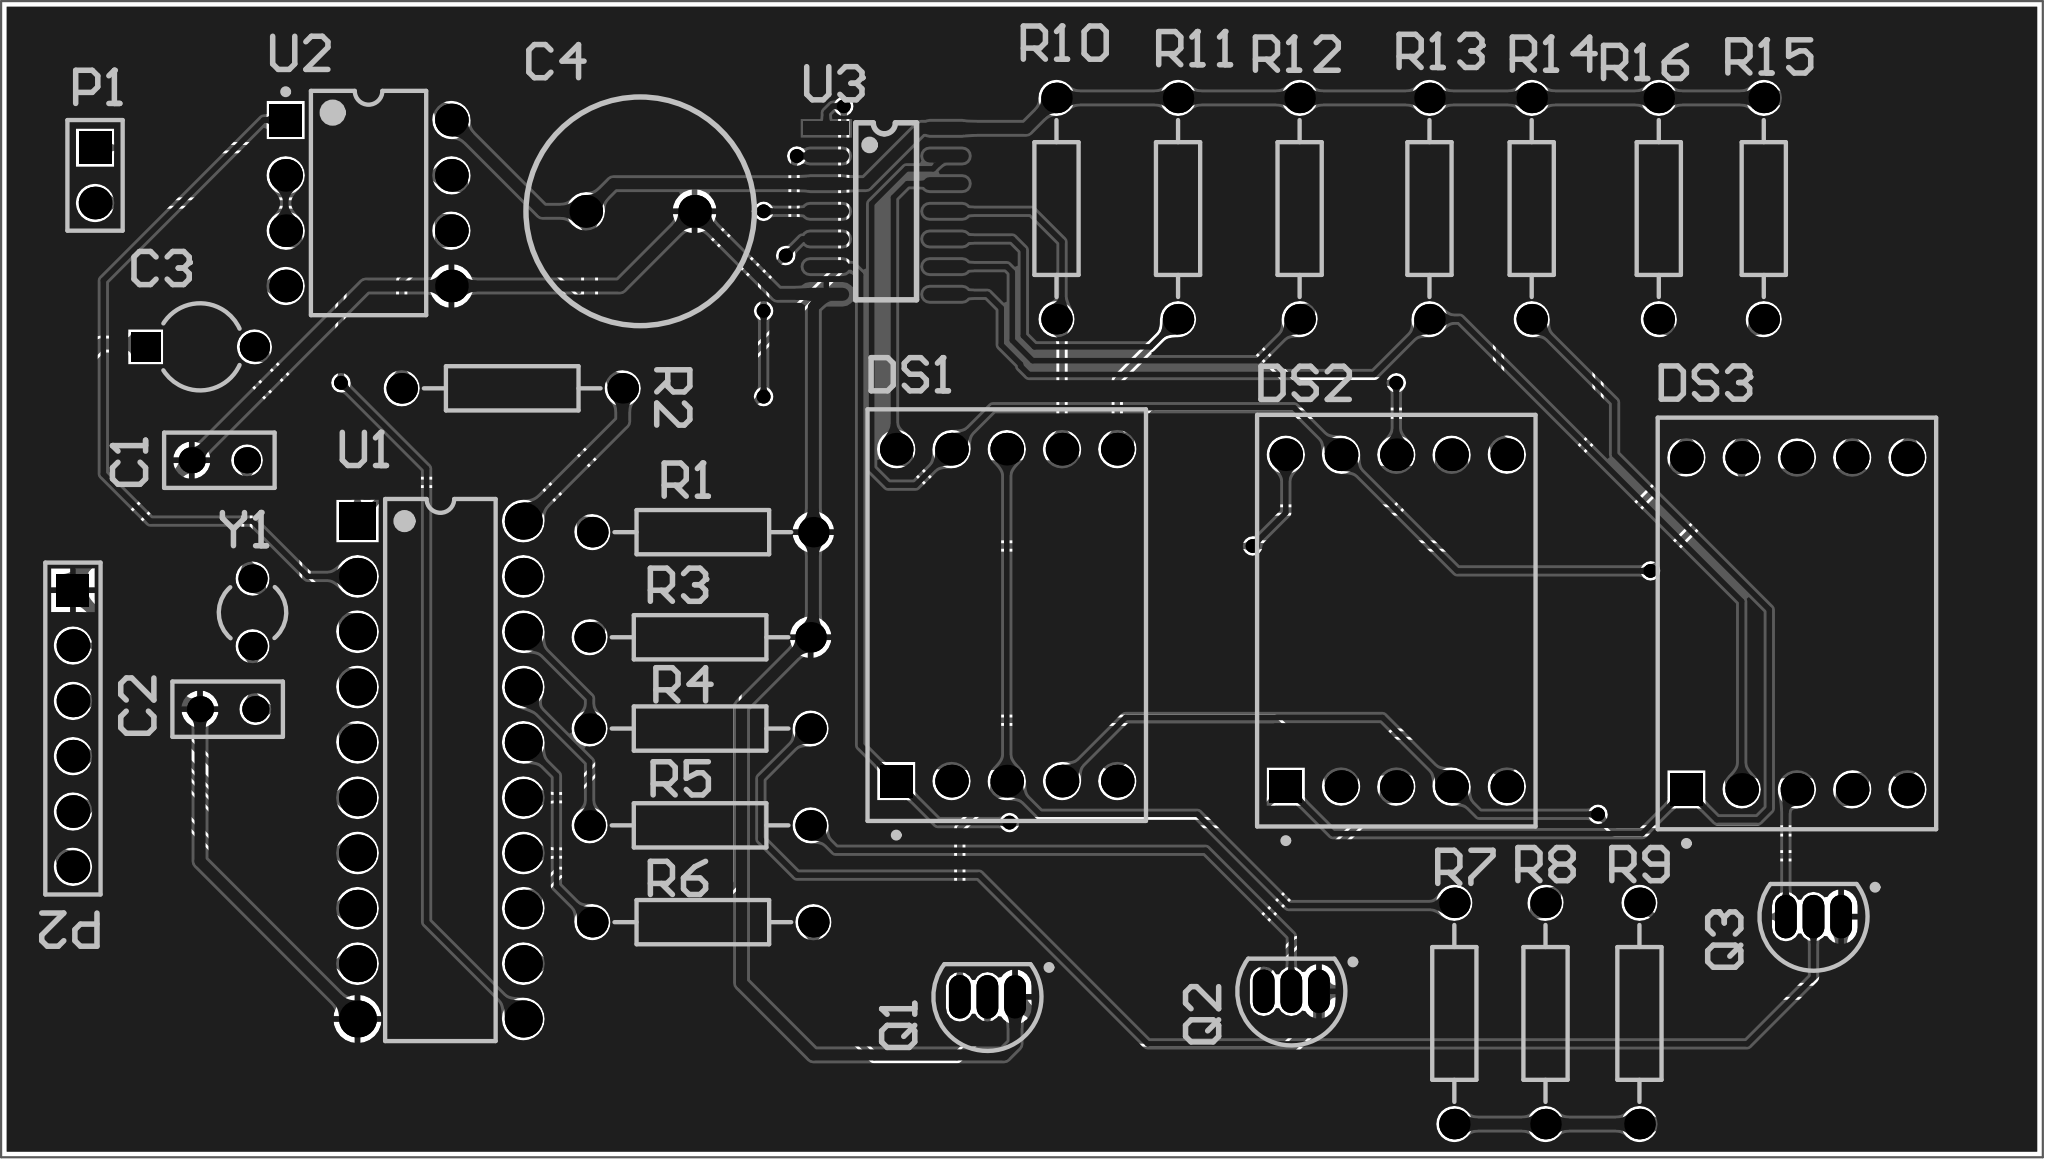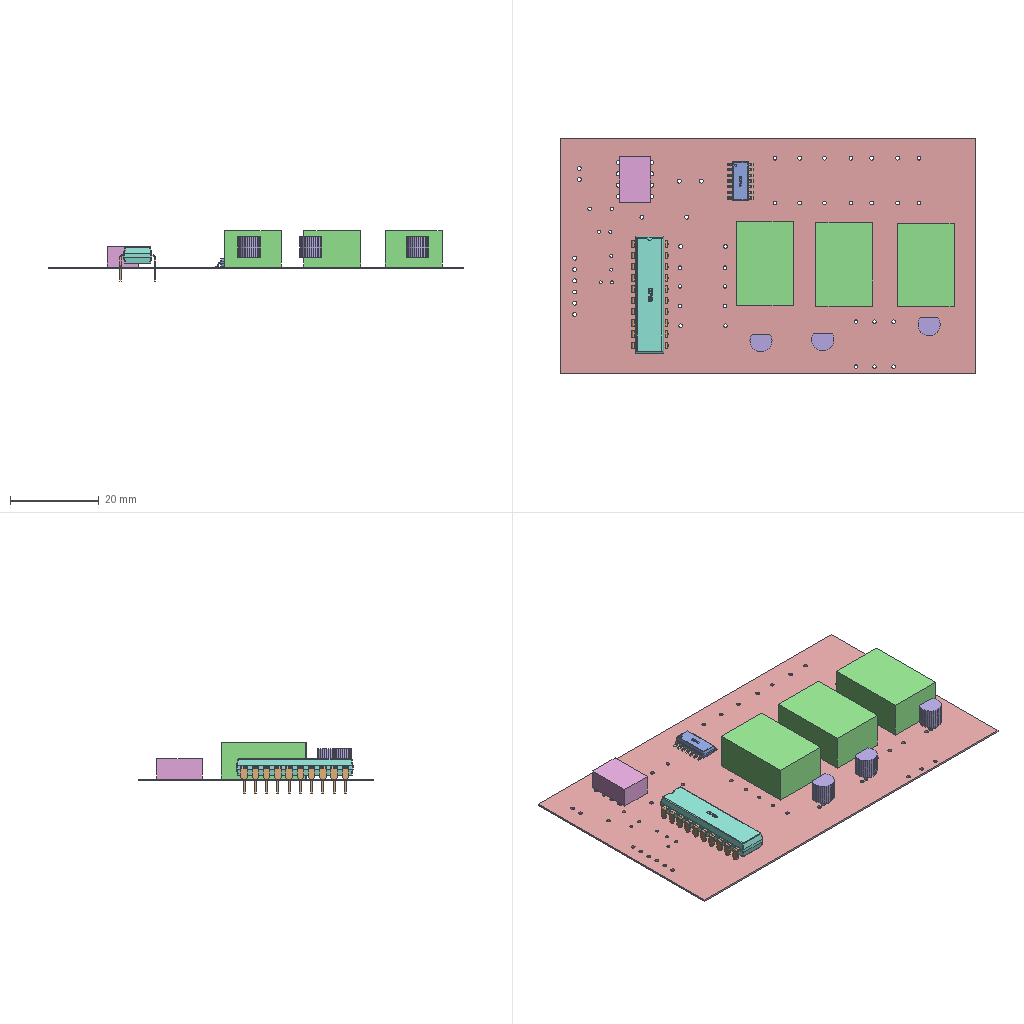Circuit board layout | Altium Designer | box 93.9 x 53.1 x 11.5 mm
Layer stack:
# Altium Designer layer stack of  (unit mm; dielectric type: 0 none, 1 core, 2 prepreg, 3 surface material)
index,name,kind,layer,copper_thickness_mm,dielectric_type,dielectric_thickness_mm,dielectric_material,dielectric_constant
0,Top Paste,other,,,,,,
1,Top Overlay,other,,,,,,
2,Top Solder,dielectric,,,3,0.0102,Solder Resist,3.5
3,Top Layer,copper,Top Layer,0.0356,,,,
4,Dielectric 1,dielectric,,,0,0.32,FR-4,4.8
5,Bottom Layer,copper,Bottom Layer,0.0356,,,,
6,Bottom Solder,dielectric,,,3,0.0102,Solder Resist,3.5
7,Bottom Overlay,other,,,,,,
8,Bottom Paste,other,,,,,,
# drill layer pairs: low layer,high layer
drill_pair,Top Layer,Bottom Layer
Part placement:
Designator,Comment,Layer,Footprint,Center-X(mm),Center-Y(mm),Rotation
Y1,XTAL,TopLayer,R38,54.61,64.135,0
U3,SN74LS49D,TopLayer,SOP14,83.737,82.55,0
U2,MAX1487EPA,TopLayer,PA8,59.944,82.931,0
U1,AT89C2051,TopLayer,DIP20,63.246,56.896,0
R16,Res2,TopLayer,AXIAL-0.4,119.253,82.677,270
R15,Res2,TopLayer,AXIAL-0.4,124.079,82.677,270
R14,Res2,TopLayer,AXIAL-0.4,113.411,82.677,270
R13,Res2,TopLayer,AXIAL-0.4,108.712,82.677,270
R12,Res2,TopLayer,AXIAL-0.4,102.743,82.677,270
R11,Res2,TopLayer,AXIAL-0.4,97.155,82.677,270
R10,Res2,TopLayer,AXIAL-0.4,91.567,82.677,270
R9,Res2,TopLayer,AXIAL-0.4,118.364,45.72,90
R8,Res2,TopLayer,AXIAL-0.4,114.046,45.72,90
R7,Res2,TopLayer,AXIAL-0.4,109.855,45.72,90
R6,Res2,TopLayer,AXIAL-0.4,75.311,49.911,180
R5,Res2,TopLayer,AXIAL-0.4,75.184,54.356,180
R4,Res2,TopLayer,AXIAL-0.4,75.184,58.801,180
R3,Res2,TopLayer,AXIAL-0.4,75.184,62.992,180
R2,Res2,TopLayer,AXIAL-0.4,66.548,74.422,360
R1,Res2,TopLayer,AXIAL-0.4,75.311,67.818,180
Q3,9013,TopLayer,TO-92A,126.365,50.165,90
Q2,9013,TopLayer,TO-92A,102.362,46.736,90
Q1,9013,TopLayer,TO-92A,88.392,46.482,90
P2,Header 6,TopLayer,HDR1X6,46.355,58.801,270
P1,Header 2,TopLayer,HDR1X2,47.371,84.201,270
DS3,Dpy Blue-CA,TopLayer,H,125.603,63.627,0
DS2,Dpy Blue-CA,TopLayer,H,107.188,63.754,0
DS1,Dpy Blue-CA,TopLayer,H,89.281,64.008,0
C4,Cap Pol2,TopLayer,RB5-10.5,72.43,82.55,0
C3,Cap Pol2,TopLayer,CAPR5-4X5,52.197,76.327,0
C2,30p,TopLayer,RAD-0.1,53.467,59.69,180
C1,30p,TopLayer,RAD-0.1,53.086,71.12,180
Pad and via stacks:
# Altium Designer via and pad stacks of  (unit mm). Each distinct definition once, with the count of objects using it.
# via: kind,start_layer,end_layer,hole_mm,diameter_mm,mode(0 simple;1 top-mid-bottom;2 full stack),diameter_per_layer,count,example_net
# pad: kind,layer,hole_mm,hole_type(0 round;1 square;2 slot),plating,top_size,top_shape(1 round;2 rect;3 octagon;9 rounded rect),mid_size,bottom_size,mode,footprint,size_per_layer,count,example
pad,Multi-Layer,0.85,0,plated,1.4x1.4,1,1.4x1.4,1.4x1.4,0,AXIAL-0.4,,32,R2.1
pad,Multi-Layer,0.9,0,plated,1.5x1.5,2,1.5x1.5,1.5x1.5,0,PA8,,1,U2.1
pad,Multi-Layer,0.9,0,plated,1.5x1.5,1,1.5x1.5,1.5x1.5,0,PA8,,7,U2.2
pad,Multi-Layer,0.9,0,plated,1.5x1.5,2,1.5x1.5,1.5x1.5,0,HDR1X2,,1,P1.1
pad,Multi-Layer,0.9,0,plated,1.5x1.5,1,1.5x1.5,1.5x1.5,0,HDR1X2,,1,P1.2
pad,Multi-Layer,0.8,0,plated,1.7x1.7,1,1.7x1.7,1.7x1.7,0,DIP20,,19,U1.11
pad,Multi-Layer,0.8,0,plated,1.7x1.7,2,1.7x1.7,1.7x1.7,0,DIP20,,1,U1.1
pad,Multi-Layer,0.9,0,plated,1.5x1.5,2,1.5x1.5,1.5x1.5,0,H,,3,DS2.1
pad,Multi-Layer,0.9,0,plated,1.5x1.5,1,1.5x1.5,1.5x1.5,0,H,,27,DS2.2
pad,Multi-Layer,0.9,0,plated,1.5x1.5,2,1.5x1.5,1.5x1.5,0,HDR1X6,,1,P2.1
pad,Multi-Layer,0.9,0,plated,1.5x1.5,1,1.5x1.5,1.5x1.5,0,HDR1X6,,5,P2.2
pad,Multi-Layer,0.8,0,plated,1.35x1.35,1,1.35x1.35,1.35x1.35,0,CAPR5-4X5,,1,C3.2
pad,Multi-Layer,0.8,0,plated,1.35x1.35,2,1.35x1.35,1.35x1.35,0,CAPR5-4X5,,1,C3.1
pad,Multi-Layer,0.9,0,plated,2x1,1,2x1,2x1,0,TO-92A,,9,Q2.3
pad,Multi-Layer,0.7,0,plated,1.3x1.3,1,1.3x1.3,1.3x1.3,0,R38,,2,Y1.1
pad,Multi-Layer,0.9,0,plated,1.5x1.5,1,1.5x1.5,1.5x1.5,0,RB5-10.5,,2,C4.1
pad,Multi-Layer,0.7,0,plated,1.2x1.2,1,1.2x1.2,1.2x1.2,0,RAD-0.1,,4,C2.1
pad,Top Layer,0,0,plated,0.6x2.1,1,0.6x2.1,0.6x2.1,0,SOP14,,13,U3.14
pad,Top Layer,0,0,plated,0.6x2.1,2,0.6x2.1,0.6x2.1,0,SOP14,,1,U3.1
via,Top Layer,Bottom Layer,0.381,0.635,0,,12,NetU1_11
Copper pours:
name,layer,net,type(0 solid;1 hatched;2 none)
Top Layer-No Net,Bottom Layer,GND,0
Top Layer-No Net,Top Layer,GND,0
Design rules, without the lines most boards share:
# Altium Designer design rules of  (exported by Altium Designer, unit mm)
# columns: name | kind | enabled | priority | scope1 | scope2 | descriptor | typed fields (field=value)
SilkToSilkClearance | 55 | enabled | 1 | All | All | Silk to Silk (Clearance=0mil) (All),(All) |
SilkToSolderMaskClearance | 54 | enabled | 1 | IsPad | All | Silk To Solder Mask (Clearance=0mil) (IsPad),(All) |
MinimumSolderMaskSliver | 53 | enabled | 1 | All | All | Minimum Solder Mask Sliver (Gap=0mil) (All),(All) |
HoleToHoleClearance | 52 | enabled | 1 | All | All | Hole To Hole Clearance (Gap=10mil) (All),(All) | gap=0.254
DiffPairsRouting | 51 | enabled | 1 | All | All | Differential Pairs Uncoupled Length using the Gap Constraints (Min=10mil) (Max=10mil) (Prefered=10mil)  and Width Constraints (Min=15mil) (Max=15mil) (Prefered=15mil) (All) |
SolderMaskExpansion | 13 | enabled | 1 | All | All | Solder Mask Expansion (Expansion =4mil) (All) | expansion=0.1016
PasteMaskExpansion | 14 | enabled | 1 | All | All | Paste Mask Expansion (Expansion =0mil) (All) | expansion=0
RoutingVias | 11 | enabled | 1 | All | All | Routing Via (MinHoleWidth=28mil) (MaxHoleWidth=28mil) (PreferredHoleWidth=28mil) (MinWidth=50mil) (MaxWidth=50mil) (PreferedWidth=50mil) (All) | via_min_hole=0.7112 via_max_hole=0.7112 via_preferred_diameter=1.27 via_preferred_hole=0.7112
Width | 2 | enabled | 1 | All | All | Width Constraint (Min=10mil) (Max=20mil) (Preferred=10mil) (All) |
PolygonConnect | 20 | enabled | 1 | All | All | Polygon Connect Rule(Relief Connect )(Conductor Width=10mil) (Relief Angle=90 Angle) (Entries=4) (Air Gap Width=10mil) (All),(All) | connect_style(0=relief,1=direct,2=none)=0 relief_conductor_width=0.254 relief_entries=4
PlaneConnect | 6 | enabled | 1 | All | All | Power Plane Connect Rule(Relief Connect )(Expansion=20mil) (Conductor Width=10mil) (Air Gap=10mil) (Entries=4) (All) | relief_conductor_width=0.254 relief_entries=4 relief_expansion=0.508
Clearance | 0 | enabled | 1 | All | All | Clearance Constraint (Gap=5mil) (All),(All) | gap=0.127